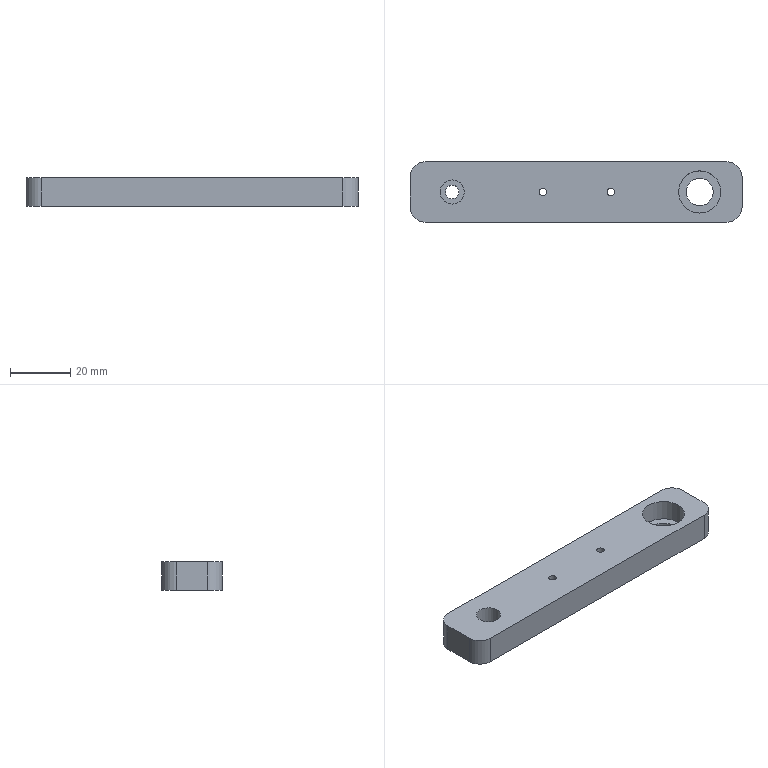Part | NX | 1 solid | 18 faces | box 110 x 20 x 9.5 mm | volume 18978 mm3 | cylinder 10 | plane 8 | commonest cylinder face diameters 10 x4 2.459 x2 4.5 x1 8 x1 9 x1 14 x1
STEP:
#1=CARTESIAN_POINT('',(11.5,-1.23,-9.5));
#2=VERTEX_POINT('',#1);
#3=CARTESIAN_POINT('',(11.5,0.,-9.5));
#4=DIRECTION('',(0.,0.,1.));
#5=DIRECTION('',(0.,-1.,0.));
#6=AXIS2_PLACEMENT_3D('',#3,#4,#5);
#7=CIRCLE('',#6,1.23);
#8=EDGE_CURVE('',#2,#2,#7,.T.);
#9=ORIENTED_EDGE('',*,*,#8,.F.);
#10=EDGE_LOOP('',(#9));
#11=FACE_BOUND('',#10,.T.);
#12=CARTESIAN_POINT('',(11.5,-1.23,0.));
#13=VERTEX_POINT('',#12);
#14=CARTESIAN_POINT('',(11.5,0.,0.));
#15=DIRECTION('',(0.,0.,1.));
#16=DIRECTION('',(0.,-1.,0.));
#17=AXIS2_PLACEMENT_3D('',#14,#15,#16);
#18=CIRCLE('',#17,1.23);
#19=EDGE_CURVE('',#13,#13,#18,.T.);
#20=ORIENTED_EDGE('',*,*,#19,.T.);
#21=EDGE_LOOP('',(#20));
#22=FACE_BOUND('',#21,.T.);
#23=CARTESIAN_POINT('',(11.5,0.,0.));
#24=DIRECTION('',(0.,0.,-1.));
#25=DIRECTION('',(0.,-1.,0.));
#26=AXIS2_PLACEMENT_3D('',#23,#24,#25);
#27=CYLINDRICAL_SURFACE('',#26,1.23);
#28=ADVANCED_FACE('',(#11,#22),#27,.F.);
#29=CARTESIAN_POINT('',(-41.,2.25,-9.5));
#30=VERTEX_POINT('',#29);
#31=CARTESIAN_POINT('',(-41.,0.,-9.5));
#32=DIRECTION('',(0.,0.,-1.));
#33=DIRECTION('',(0.,1.,0.));
#34=AXIS2_PLACEMENT_3D('',#31,#32,#33);
#35=CIRCLE('',#34,2.25);
#36=EDGE_CURVE('',#30,#30,#35,.T.);
#37=ORIENTED_EDGE('',*,*,#36,.F.);
#38=EDGE_LOOP('',(#37));
#39=FACE_BOUND('',#38,.T.);
#40=CARTESIAN_POINT('',(41.,4.5,-9.5));
#41=VERTEX_POINT('',#40);
#42=CARTESIAN_POINT('',(41.,0.,-9.5));
#43=DIRECTION('',(0.,0.,-1.));
#44=DIRECTION('',(0.,1.,0.));
#45=AXIS2_PLACEMENT_3D('',#42,#43,#44);
#46=CIRCLE('',#45,4.5);
#47=EDGE_CURVE('',#41,#41,#46,.T.);
#48=ORIENTED_EDGE('',*,*,#47,.F.);
#49=EDGE_LOOP('',(#48));
#50=FACE_BOUND('',#49,.T.);
#51=CARTESIAN_POINT('',(-11.,1.23,-9.5));
#52=VERTEX_POINT('',#51);
#53=CARTESIAN_POINT('',(-11.,0.,-9.5));
#54=DIRECTION('',(0.,0.,-1.));
#55=DIRECTION('',(0.,1.,0.));
#56=AXIS2_PLACEMENT_3D('',#53,#54,#55);
#57=CIRCLE('',#56,1.23);
#58=EDGE_CURVE('',#52,#52,#57,.T.);
#59=ORIENTED_EDGE('',*,*,#58,.F.);
#60=EDGE_LOOP('',(#59));
#61=FACE_BOUND('',#60,.T.);
#62=ORIENTED_EDGE('',*,*,#8,.T.);
#63=EDGE_LOOP('',(#62));
#64=FACE_BOUND('',#63,.T.);
#65=CARTESIAN_POINT('',(-50.,10.,-9.5));
#66=VERTEX_POINT('',#65);
#67=CARTESIAN_POINT('',(-55.,5.,-9.5));
#68=VERTEX_POINT('',#67);
#69=CARTESIAN_POINT('',(-50.,5.,-9.5));
#70=DIRECTION('',(0.,0.,1.));
#71=DIRECTION('',(0.,-1.,0.));
#72=AXIS2_PLACEMENT_3D('',#69,#70,#71);
#73=CIRCLE('',#72,5.);
#74=EDGE_CURVE('',#66,#68,#73,.T.);
#75=ORIENTED_EDGE('',*,*,#74,.F.);
#76=CARTESIAN_POINT('',(50.,10.,-9.5));
#77=VERTEX_POINT('',#76);
#78=CARTESIAN_POINT('',(0.,10.,-9.5));
#79=DIRECTION('',(1.,0.,0.));
#80=VECTOR('',#79,1000.);
#81=LINE('',#78,#80);
#82=EDGE_CURVE('',#66,#77,#81,.T.);
#83=ORIENTED_EDGE('',*,*,#82,.T.);
#84=CARTESIAN_POINT('',(55.,5.,-9.5));
#85=VERTEX_POINT('',#84);
#86=CARTESIAN_POINT('',(50.,5.,-9.5));
#87=DIRECTION('',(0.,0.,1.));
#88=DIRECTION('',(0.,-1.,0.));
#89=AXIS2_PLACEMENT_3D('',#86,#87,#88);
#90=CIRCLE('',#89,5.);
#91=EDGE_CURVE('',#85,#77,#90,.T.);
#92=ORIENTED_EDGE('',*,*,#91,.F.);
#93=CARTESIAN_POINT('',(55.,-5.,-9.5));
#94=VERTEX_POINT('',#93);
#95=CARTESIAN_POINT('',(55.,0.,-9.5));
#96=DIRECTION('',(0.,-1.,0.));
#97=VECTOR('',#96,1000.);
#98=LINE('',#95,#97);
#99=EDGE_CURVE('',#85,#94,#98,.T.);
#100=ORIENTED_EDGE('',*,*,#99,.T.);
#101=CARTESIAN_POINT('',(50.,-10.,-9.5));
#102=VERTEX_POINT('',#101);
#103=CARTESIAN_POINT('',(50.,-5.,-9.5));
#104=DIRECTION('',(0.,0.,1.));
#105=DIRECTION('',(0.,-1.,0.));
#106=AXIS2_PLACEMENT_3D('',#103,#104,#105);
#107=CIRCLE('',#106,5.);
#108=EDGE_CURVE('',#102,#94,#107,.T.);
#109=ORIENTED_EDGE('',*,*,#108,.F.);
#110=CARTESIAN_POINT('',(-50.,-10.,-9.5));
#111=VERTEX_POINT('',#110);
#112=CARTESIAN_POINT('',(0.,-10.,-9.5));
#113=DIRECTION('',(-1.,0.,0.));
#114=VECTOR('',#113,1000.);
#115=LINE('',#112,#114);
#116=EDGE_CURVE('',#102,#111,#115,.T.);
#117=ORIENTED_EDGE('',*,*,#116,.T.);
#118=CARTESIAN_POINT('',(-55.,-5.,-9.5));
#119=VERTEX_POINT('',#118);
#120=CARTESIAN_POINT('',(-50.,-5.,-9.5));
#121=DIRECTION('',(0.,0.,1.));
#122=DIRECTION('',(0.,-1.,0.));
#123=AXIS2_PLACEMENT_3D('',#120,#121,#122);
#124=CIRCLE('',#123,5.);
#125=EDGE_CURVE('',#119,#111,#124,.T.);
#126=ORIENTED_EDGE('',*,*,#125,.F.);
#127=CARTESIAN_POINT('',(-55.,0.,-9.5));
#128=DIRECTION('',(0.,1.,0.));
#129=VECTOR('',#128,1000.);
#130=LINE('',#127,#129);
#131=EDGE_CURVE('',#119,#68,#130,.T.);
#132=ORIENTED_EDGE('',*,*,#131,.T.);
#133=EDGE_LOOP('',(#75,#83,#92,#100,#109,#117,#126,#132));
#134=FACE_BOUND('',#133,.T.);
#135=CARTESIAN_POINT('',(0.,0.,-9.5));
#136=DIRECTION('',(0.,0.,1.));
#137=DIRECTION('',(0.,-1.,0.));
#138=AXIS2_PLACEMENT_3D('',#135,#136,#137);
#139=PLANE('',#138);
#140=ADVANCED_FACE('',(#39,#50,#61,#64,#134),#139,.F.);
#141=CARTESIAN_POINT('',(-55.,-5.,0.));
#142=VERTEX_POINT('',#141);
#143=CARTESIAN_POINT('',(-50.,-10.,0.));
#144=VERTEX_POINT('',#143);
#145=CARTESIAN_POINT('',(-50.,-5.,0.));
#146=DIRECTION('',(0.,0.,1.));
#147=DIRECTION('',(0.,-1.,0.));
#148=AXIS2_PLACEMENT_3D('',#145,#146,#147);
#149=CIRCLE('',#148,5.);
#150=EDGE_CURVE('',#142,#144,#149,.T.);
#151=ORIENTED_EDGE('',*,*,#150,.F.);
#152=CARTESIAN_POINT('',(-55.,-5.,-4.75));
#153=DIRECTION('',(0.,0.,1.));
#154=VECTOR('',#153,1000.);
#155=LINE('',#152,#154);
#156=EDGE_CURVE('',#119,#142,#155,.T.);
#157=ORIENTED_EDGE('',*,*,#156,.F.);
#158=ORIENTED_EDGE('',*,*,#125,.T.);
#159=CARTESIAN_POINT('',(-50.,-10.,-4.75));
#160=DIRECTION('',(0.,0.,1.));
#161=VECTOR('',#160,1000.);
#162=LINE('',#159,#161);
#163=EDGE_CURVE('',#111,#144,#162,.T.);
#164=ORIENTED_EDGE('',*,*,#163,.T.);
#165=EDGE_LOOP('',(#151,#157,#158,#164));
#166=FACE_BOUND('',#165,.T.);
#167=CARTESIAN_POINT('',(-50.,-5.,-4.75));
#168=DIRECTION('',(0.,0.,1.));
#169=DIRECTION('',(-1.,0.,0.));
#170=AXIS2_PLACEMENT_3D('',#167,#168,#169);
#171=CYLINDRICAL_SURFACE('',#170,5.);
#172=ADVANCED_FACE('',(#166),#171,.T.);
#173=CARTESIAN_POINT('',(50.,-10.,0.));
#174=VERTEX_POINT('',#173);
#175=CARTESIAN_POINT('',(55.,-5.,0.));
#176=VERTEX_POINT('',#175);
#177=CARTESIAN_POINT('',(50.,-5.,0.));
#178=DIRECTION('',(0.,0.,1.));
#179=DIRECTION('',(0.,-1.,0.));
#180=AXIS2_PLACEMENT_3D('',#177,#178,#179);
#181=CIRCLE('',#180,5.);
#182=EDGE_CURVE('',#174,#176,#181,.T.);
#183=ORIENTED_EDGE('',*,*,#182,.F.);
#184=CARTESIAN_POINT('',(50.,-10.,-4.75));
#185=DIRECTION('',(0.,0.,1.));
#186=VECTOR('',#185,1000.);
#187=LINE('',#184,#186);
#188=EDGE_CURVE('',#102,#174,#187,.T.);
#189=ORIENTED_EDGE('',*,*,#188,.F.);
#190=ORIENTED_EDGE('',*,*,#108,.T.);
#191=CARTESIAN_POINT('',(55.,-5.,-4.75));
#192=DIRECTION('',(0.,0.,1.));
#193=VECTOR('',#192,1000.);
#194=LINE('',#191,#193);
#195=EDGE_CURVE('',#94,#176,#194,.T.);
#196=ORIENTED_EDGE('',*,*,#195,.T.);
#197=EDGE_LOOP('',(#183,#189,#190,#196));
#198=FACE_BOUND('',#197,.T.);
#199=CARTESIAN_POINT('',(50.,-5.,-4.75));
#200=DIRECTION('',(0.,0.,1.));
#201=DIRECTION('',(0.,-1.,0.));
#202=AXIS2_PLACEMENT_3D('',#199,#200,#201);
#203=CYLINDRICAL_SURFACE('',#202,5.);
#204=ADVANCED_FACE('',(#198),#203,.T.);
#205=CARTESIAN_POINT('',(55.,5.,0.));
#206=VERTEX_POINT('',#205);
#207=CARTESIAN_POINT('',(50.,10.,0.));
#208=VERTEX_POINT('',#207);
#209=CARTESIAN_POINT('',(50.,5.,0.));
#210=DIRECTION('',(0.,0.,1.));
#211=DIRECTION('',(0.,-1.,0.));
#212=AXIS2_PLACEMENT_3D('',#209,#210,#211);
#213=CIRCLE('',#212,5.);
#214=EDGE_CURVE('',#206,#208,#213,.T.);
#215=ORIENTED_EDGE('',*,*,#214,.F.);
#216=CARTESIAN_POINT('',(55.,5.,-4.75));
#217=DIRECTION('',(0.,0.,1.));
#218=VECTOR('',#217,1000.);
#219=LINE('',#216,#218);
#220=EDGE_CURVE('',#85,#206,#219,.T.);
#221=ORIENTED_EDGE('',*,*,#220,.F.);
#222=ORIENTED_EDGE('',*,*,#91,.T.);
#223=CARTESIAN_POINT('',(50.,10.,-4.75));
#224=DIRECTION('',(0.,0.,1.));
#225=VECTOR('',#224,1000.);
#226=LINE('',#223,#225);
#227=EDGE_CURVE('',#77,#208,#226,.T.);
#228=ORIENTED_EDGE('',*,*,#227,.T.);
#229=EDGE_LOOP('',(#215,#221,#222,#228));
#230=FACE_BOUND('',#229,.T.);
#231=CARTESIAN_POINT('',(50.,5.,-4.75));
#232=DIRECTION('',(0.,0.,1.));
#233=DIRECTION('',(1.,0.,0.));
#234=AXIS2_PLACEMENT_3D('',#231,#232,#233);
#235=CYLINDRICAL_SURFACE('',#234,5.);
#236=ADVANCED_FACE('',(#230),#235,.T.);
#237=CARTESIAN_POINT('',(-50.,10.,0.));
#238=VERTEX_POINT('',#237);
#239=CARTESIAN_POINT('',(-55.,5.,0.));
#240=VERTEX_POINT('',#239);
#241=CARTESIAN_POINT('',(-50.,5.,0.));
#242=DIRECTION('',(0.,0.,1.));
#243=DIRECTION('',(0.,-1.,0.));
#244=AXIS2_PLACEMENT_3D('',#241,#242,#243);
#245=CIRCLE('',#244,5.);
#246=EDGE_CURVE('',#238,#240,#245,.T.);
#247=ORIENTED_EDGE('',*,*,#246,.F.);
#248=CARTESIAN_POINT('',(-50.,10.,-4.75));
#249=DIRECTION('',(0.,0.,1.));
#250=VECTOR('',#249,1000.);
#251=LINE('',#248,#250);
#252=EDGE_CURVE('',#66,#238,#251,.T.);
#253=ORIENTED_EDGE('',*,*,#252,.F.);
#254=ORIENTED_EDGE('',*,*,#74,.T.);
#255=CARTESIAN_POINT('',(-55.,5.,-4.75));
#256=DIRECTION('',(0.,0.,1.));
#257=VECTOR('',#256,1000.);
#258=LINE('',#255,#257);
#259=EDGE_CURVE('',#68,#240,#258,.T.);
#260=ORIENTED_EDGE('',*,*,#259,.T.);
#261=EDGE_LOOP('',(#247,#253,#254,#260));
#262=FACE_BOUND('',#261,.T.);
#263=CARTESIAN_POINT('',(-50.,5.,-4.75));
#264=DIRECTION('',(0.,0.,1.));
#265=DIRECTION('',(0.,1.,0.));
#266=AXIS2_PLACEMENT_3D('',#263,#264,#265);
#267=CYLINDRICAL_SURFACE('',#266,5.);
#268=ADVANCED_FACE('',(#262),#267,.T.);
#269=CARTESIAN_POINT('',(41.,7.,-7.));
#270=VERTEX_POINT('',#269);
#271=CARTESIAN_POINT('',(41.,0.,-7.));
#272=DIRECTION('',(0.,0.,-1.));
#273=DIRECTION('',(0.,1.,0.));
#274=AXIS2_PLACEMENT_3D('',#271,#272,#273);
#275=CIRCLE('',#274,7.);
#276=EDGE_CURVE('',#270,#270,#275,.T.);
#277=ORIENTED_EDGE('',*,*,#276,.T.);
#278=EDGE_LOOP('',(#277));
#279=FACE_BOUND('',#278,.T.);
#280=CARTESIAN_POINT('',(41.,-7.,0.));
#281=VERTEX_POINT('',#280);
#282=CARTESIAN_POINT('',(41.,0.,0.));
#283=DIRECTION('',(0.,0.,1.));
#284=DIRECTION('',(0.,-1.,0.));
#285=AXIS2_PLACEMENT_3D('',#282,#283,#284);
#286=CIRCLE('',#285,7.);
#287=EDGE_CURVE('',#281,#281,#286,.T.);
#288=ORIENTED_EDGE('',*,*,#287,.T.);
#289=EDGE_LOOP('',(#288));
#290=FACE_BOUND('',#289,.T.);
#291=CARTESIAN_POINT('',(41.,0.,0.));
#292=DIRECTION('',(0.,0.,-1.));
#293=DIRECTION('',(0.,-1.,0.));
#294=AXIS2_PLACEMENT_3D('',#291,#292,#293);
#295=CYLINDRICAL_SURFACE('',#294,7.);
#296=ADVANCED_FACE('',(#279,#290),#295,.F.);
#297=CARTESIAN_POINT('',(-41.,4.,-7.));
#298=VERTEX_POINT('',#297);
#299=CARTESIAN_POINT('',(-41.,0.,-7.));
#300=DIRECTION('',(0.,0.,-1.));
#301=DIRECTION('',(0.,1.,0.));
#302=AXIS2_PLACEMENT_3D('',#299,#300,#301);
#303=CIRCLE('',#302,4.);
#304=EDGE_CURVE('',#298,#298,#303,.T.);
#305=ORIENTED_EDGE('',*,*,#304,.T.);
#306=EDGE_LOOP('',(#305));
#307=FACE_BOUND('',#306,.T.);
#308=CARTESIAN_POINT('',(-41.,-4.,0.));
#309=VERTEX_POINT('',#308);
#310=CARTESIAN_POINT('',(-41.,0.,0.));
#311=DIRECTION('',(0.,0.,1.));
#312=DIRECTION('',(0.,-1.,0.));
#313=AXIS2_PLACEMENT_3D('',#310,#311,#312);
#314=CIRCLE('',#313,4.);
#315=EDGE_CURVE('',#309,#309,#314,.T.);
#316=ORIENTED_EDGE('',*,*,#315,.T.);
#317=EDGE_LOOP('',(#316));
#318=FACE_BOUND('',#317,.T.);
#319=CARTESIAN_POINT('',(-41.,0.,0.));
#320=DIRECTION('',(0.,0.,-1.));
#321=DIRECTION('',(0.,-1.,0.));
#322=AXIS2_PLACEMENT_3D('',#319,#320,#321);
#323=CYLINDRICAL_SURFACE('',#322,4.);
#324=ADVANCED_FACE('',(#307,#318),#323,.F.);
#325=CARTESIAN_POINT('',(41.,4.5,-7.));
#326=VERTEX_POINT('',#325);
#327=CARTESIAN_POINT('',(41.,0.,-7.));
#328=DIRECTION('',(0.,0.,-1.));
#329=DIRECTION('',(0.,1.,0.));
#330=AXIS2_PLACEMENT_3D('',#327,#328,#329);
#331=CIRCLE('',#330,4.5);
#332=EDGE_CURVE('',#326,#326,#331,.T.);
#333=ORIENTED_EDGE('',*,*,#332,.T.);
#334=EDGE_LOOP('',(#333));
#335=FACE_BOUND('',#334,.T.);
#336=ORIENTED_EDGE('',*,*,#276,.F.);
#337=EDGE_LOOP('',(#336));
#338=FACE_BOUND('',#337,.T.);
#339=CARTESIAN_POINT('',(-41.,-2.25,-7.));
#340=DIRECTION('',(0.,0.,-1.));
#341=DIRECTION('',(0.,-1.,0.));
#342=AXIS2_PLACEMENT_3D('',#339,#340,#341);
#343=PLANE('',#342);
#344=ADVANCED_FACE('',(#335,#338),#343,.F.);
#345=CARTESIAN_POINT('',(-41.,2.25,-7.));
#346=VERTEX_POINT('',#345);
#347=CARTESIAN_POINT('',(-41.,0.,-7.));
#348=DIRECTION('',(0.,0.,-1.));
#349=DIRECTION('',(0.,1.,0.));
#350=AXIS2_PLACEMENT_3D('',#347,#348,#349);
#351=CIRCLE('',#350,2.25);
#352=EDGE_CURVE('',#346,#346,#351,.T.);
#353=ORIENTED_EDGE('',*,*,#352,.T.);
#354=EDGE_LOOP('',(#353));
#355=FACE_BOUND('',#354,.T.);
#356=ORIENTED_EDGE('',*,*,#304,.F.);
#357=EDGE_LOOP('',(#356));
#358=FACE_BOUND('',#357,.T.);
#359=CARTESIAN_POINT('',(-41.,-2.25,-7.));
#360=DIRECTION('',(0.,0.,-1.));
#361=DIRECTION('',(0.,-1.,0.));
#362=AXIS2_PLACEMENT_3D('',#359,#360,#361);
#363=PLANE('',#362);
#364=ADVANCED_FACE('',(#355,#358),#363,.F.);
#365=ORIENTED_EDGE('',*,*,#36,.T.);
#366=EDGE_LOOP('',(#365));
#367=FACE_BOUND('',#366,.T.);
#368=ORIENTED_EDGE('',*,*,#352,.F.);
#369=EDGE_LOOP('',(#368));
#370=FACE_BOUND('',#369,.T.);
#371=CARTESIAN_POINT('',(-41.,0.,0.));
#372=DIRECTION('',(0.,0.,-1.));
#373=DIRECTION('',(0.,-1.,0.));
#374=AXIS2_PLACEMENT_3D('',#371,#372,#373);
#375=CYLINDRICAL_SURFACE('',#374,2.25);
#376=ADVANCED_FACE('',(#367,#370),#375,.F.);
#377=ORIENTED_EDGE('',*,*,#47,.T.);
#378=EDGE_LOOP('',(#377));
#379=FACE_BOUND('',#378,.T.);
#380=ORIENTED_EDGE('',*,*,#332,.F.);
#381=EDGE_LOOP('',(#380));
#382=FACE_BOUND('',#381,.T.);
#383=CARTESIAN_POINT('',(41.,0.,0.));
#384=DIRECTION('',(0.,0.,-1.));
#385=DIRECTION('',(0.,-1.,0.));
#386=AXIS2_PLACEMENT_3D('',#383,#384,#385);
#387=CYLINDRICAL_SURFACE('',#386,4.5);
#388=ADVANCED_FACE('',(#379,#382),#387,.F.);
#389=ORIENTED_EDGE('',*,*,#252,.T.);
#390=CARTESIAN_POINT('',(0.,10.,0.));
#391=DIRECTION('',(1.,0.,0.));
#392=VECTOR('',#391,1000.);
#393=LINE('',#390,#392);
#394=EDGE_CURVE('',#238,#208,#393,.T.);
#395=ORIENTED_EDGE('',*,*,#394,.T.);
#396=ORIENTED_EDGE('',*,*,#227,.F.);
#397=ORIENTED_EDGE('',*,*,#82,.F.);
#398=EDGE_LOOP('',(#389,#395,#396,#397));
#399=FACE_BOUND('',#398,.T.);
#400=CARTESIAN_POINT('',(-55.,10.,-9.5));
#401=DIRECTION('',(0.,-1.,0.));
#402=DIRECTION('',(1.,0.,0.));
#403=AXIS2_PLACEMENT_3D('',#400,#401,#402);
#404=PLANE('',#403);
#405=ADVANCED_FACE('',(#399),#404,.F.);
#406=ORIENTED_EDGE('',*,*,#220,.T.);
#407=CARTESIAN_POINT('',(55.,0.,0.));
#408=DIRECTION('',(0.,-1.,0.));
#409=VECTOR('',#408,1000.);
#410=LINE('',#407,#409);
#411=EDGE_CURVE('',#206,#176,#410,.T.);
#412=ORIENTED_EDGE('',*,*,#411,.T.);
#413=ORIENTED_EDGE('',*,*,#195,.F.);
#414=ORIENTED_EDGE('',*,*,#99,.F.);
#415=EDGE_LOOP('',(#406,#412,#413,#414));
#416=FACE_BOUND('',#415,.T.);
#417=CARTESIAN_POINT('',(55.,10.,-9.5));
#418=DIRECTION('',(-1.,0.,0.));
#419=DIRECTION('',(0.,-1.,0.));
#420=AXIS2_PLACEMENT_3D('',#417,#418,#419);
#421=PLANE('',#420);
#422=ADVANCED_FACE('',(#416),#421,.F.);
#423=ORIENTED_EDGE('',*,*,#163,.F.);
#424=ORIENTED_EDGE('',*,*,#116,.F.);
#425=ORIENTED_EDGE('',*,*,#188,.T.);
#426=CARTESIAN_POINT('',(0.,-10.,0.));
#427=DIRECTION('',(-1.,0.,0.));
#428=VECTOR('',#427,1000.);
#429=LINE('',#426,#428);
#430=EDGE_CURVE('',#174,#144,#429,.T.);
#431=ORIENTED_EDGE('',*,*,#430,.T.);
#432=EDGE_LOOP('',(#423,#424,#425,#431));
#433=FACE_BOUND('',#432,.T.);
#434=CARTESIAN_POINT('',(55.,-10.,-9.5));
#435=DIRECTION('',(0.,1.,0.));
#436=DIRECTION('',(-1.,0.,0.));
#437=AXIS2_PLACEMENT_3D('',#434,#435,#436);
#438=PLANE('',#437);
#439=ADVANCED_FACE('',(#433),#438,.F.);
#440=ORIENTED_EDGE('',*,*,#259,.F.);
#441=ORIENTED_EDGE('',*,*,#131,.F.);
#442=ORIENTED_EDGE('',*,*,#156,.T.);
#443=CARTESIAN_POINT('',(-55.,0.,0.));
#444=DIRECTION('',(0.,1.,0.));
#445=VECTOR('',#444,1000.);
#446=LINE('',#443,#445);
#447=EDGE_CURVE('',#142,#240,#446,.T.);
#448=ORIENTED_EDGE('',*,*,#447,.T.);
#449=EDGE_LOOP('',(#440,#441,#442,#448));
#450=FACE_BOUND('',#449,.T.);
#451=CARTESIAN_POINT('',(-55.,-10.,-9.5));
#452=DIRECTION('',(1.,0.,0.));
#453=DIRECTION('',(0.,1.,0.));
#454=AXIS2_PLACEMENT_3D('',#451,#452,#453);
#455=PLANE('',#454);
#456=ADVANCED_FACE('',(#450),#455,.F.);
#457=ORIENTED_EDGE('',*,*,#315,.F.);
#458=EDGE_LOOP('',(#457));
#459=FACE_BOUND('',#458,.T.);
#460=ORIENTED_EDGE('',*,*,#287,.F.);
#461=EDGE_LOOP('',(#460));
#462=FACE_BOUND('',#461,.T.);
#463=CARTESIAN_POINT('',(-11.,1.23,0.));
#464=VERTEX_POINT('',#463);
#465=CARTESIAN_POINT('',(-11.,0.,0.));
#466=DIRECTION('',(0.,0.,-1.));
#467=DIRECTION('',(0.,1.,0.));
#468=AXIS2_PLACEMENT_3D('',#465,#466,#467);
#469=CIRCLE('',#468,1.23);
#470=EDGE_CURVE('',#464,#464,#469,.T.);
#471=ORIENTED_EDGE('',*,*,#470,.T.);
#472=EDGE_LOOP('',(#471));
#473=FACE_BOUND('',#472,.T.);
#474=ORIENTED_EDGE('',*,*,#19,.F.);
#475=EDGE_LOOP('',(#474));
#476=FACE_BOUND('',#475,.T.);
#477=ORIENTED_EDGE('',*,*,#447,.F.);
#478=ORIENTED_EDGE('',*,*,#150,.T.);
#479=ORIENTED_EDGE('',*,*,#430,.F.);
#480=ORIENTED_EDGE('',*,*,#182,.T.);
#481=ORIENTED_EDGE('',*,*,#411,.F.);
#482=ORIENTED_EDGE('',*,*,#214,.T.);
#483=ORIENTED_EDGE('',*,*,#394,.F.);
#484=ORIENTED_EDGE('',*,*,#246,.T.);
#485=EDGE_LOOP('',(#477,#478,#479,#480,#481,#482,#483,#484));
#486=FACE_BOUND('',#485,.T.);
#487=CARTESIAN_POINT('',(0.,0.,0.));
#488=DIRECTION('',(0.,0.,1.));
#489=DIRECTION('',(0.,-1.,0.));
#490=AXIS2_PLACEMENT_3D('',#487,#488,#489);
#491=PLANE('',#490);
#492=ADVANCED_FACE('',(#459,#462,#473,#476,#486),#491,.T.);
#493=ORIENTED_EDGE('',*,*,#58,.T.);
#494=EDGE_LOOP('',(#493));
#495=FACE_BOUND('',#494,.T.);
#496=ORIENTED_EDGE('',*,*,#470,.F.);
#497=EDGE_LOOP('',(#496));
#498=FACE_BOUND('',#497,.T.);
#499=CARTESIAN_POINT('',(-11.,0.,0.));
#500=DIRECTION('',(0.,0.,-1.));
#501=DIRECTION('',(0.,-1.,0.));
#502=AXIS2_PLACEMENT_3D('',#499,#500,#501);
#503=CYLINDRICAL_SURFACE('',#502,1.23);
#504=ADVANCED_FACE('',(#495,#498),#503,.F.);
#505=CLOSED_SHELL('',(#28,#140,#172,#204,#236,#268,#296,#324,#344,#364,#376,#388,#405,#422,#439,#456,#492,#504));
#506=MANIFOLD_SOLID_BREP('',#505);
#507=(LENGTH_UNIT()NAMED_UNIT(*)SI_UNIT(.MILLI.,.METRE.));
#508=UNCERTAINTY_MEASURE_WITH_UNIT(LENGTH_MEASURE(0.00001),#507,'','');
#509=(NAMED_UNIT(*)PLANE_ANGLE_UNIT()SI_UNIT($,.RADIAN.));
#510=(NAMED_UNIT(*)SI_UNIT($,.STERADIAN.)SOLID_ANGLE_UNIT());
#511=(GEOMETRIC_REPRESENTATION_CONTEXT(3)GLOBAL_UNCERTAINTY_ASSIGNED_CONTEXT((#508))GLOBAL_UNIT_ASSIGNED_CONTEXT((#507,#509,#510))REPRESENTATION_CONTEXT('',''));
#512=ADVANCED_BREP_SHAPE_REPRESENTATION('',(#506),#511);